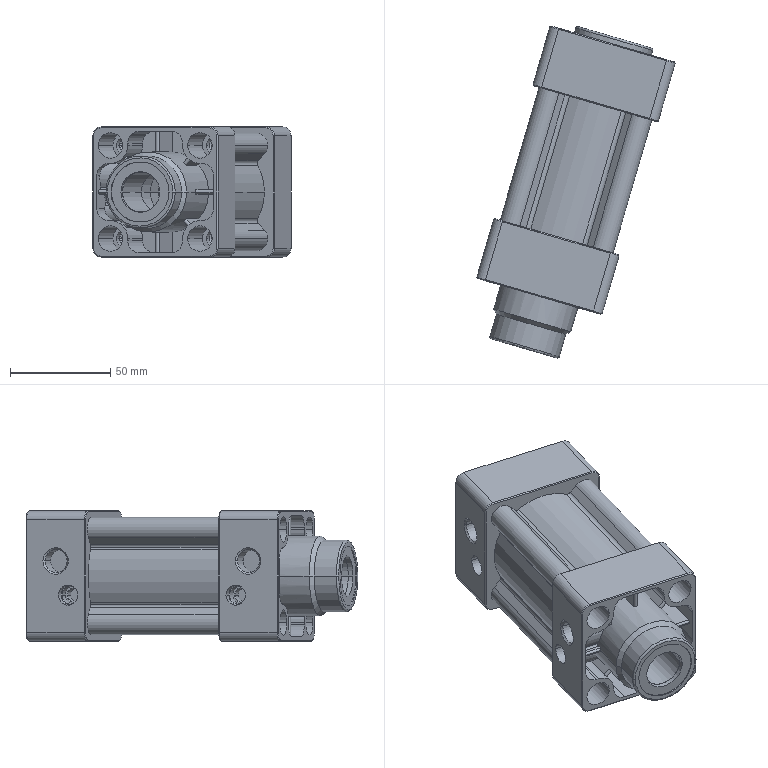Part | SolidWorks | features BaseBody 1 | 1 solid | 355 faces | box 98.795 x 165.44 x 65 mm | volume 242429 mm3 | cylinder 167 | plane 138 | cone 46 | spline 4 | commonest cylinder face diameters 2 x27 12 x22 8.7 x16 12.7 x16 4 x10 6.8 x8